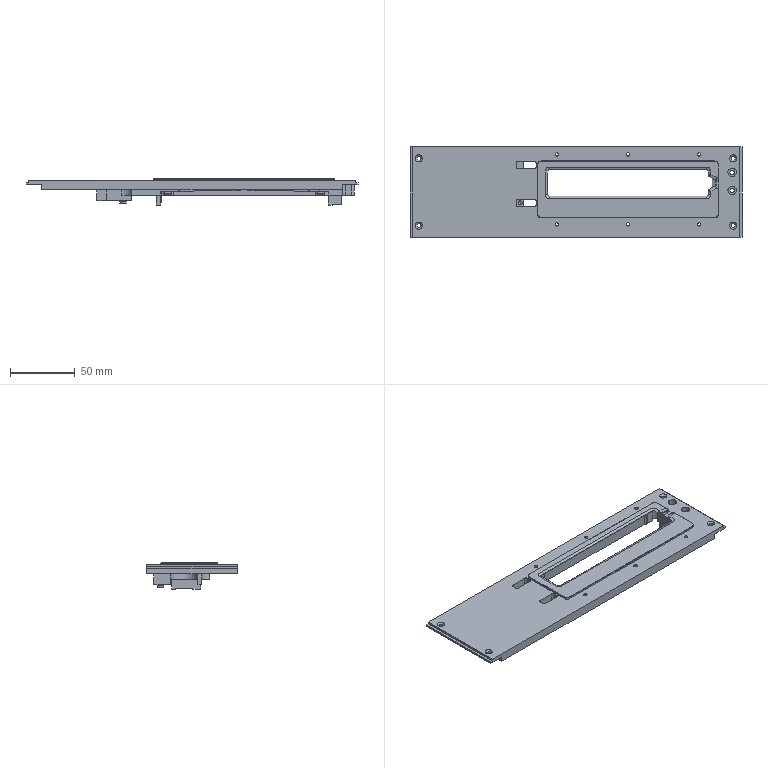NC program | NX | posted with a generic post | part box 256.6 x 70.3 x 20.422 mm
Lines 5836 to 6737 of 23702:
(CAVITY_MILL_COPY_COPY , TOOL : D4)
N11658 T04 M6
N11660 G54
N11662 G17 G0 G90 X21.865 Y-0.04 S9500 M3
N11664 G43 Z30. H4
N11666 Z-0.118
N11668 G94 G1 Z-1.118 F1000.
N11670 G3 X22.479 Y0.418 R1.
N11672 G2 X22.913 Y0.929 R2. F1400.
N11674 G1 Y1.639
N11676 G3 X22.513 Y2.439 R1.
N11678 G1 Z-0.118
N11680 G0 X21.816 Y-0.307 Z-0.32
N11682 G1 Z-1.32 F1000.
N11684 G3 X22.374 Y0.218 R1.
N11686 G2 X22.708 Y0.731 R2. F1400.
N11688 G1 Y1.369
N11690 G3 X22.308 Y2.169 R1.
N11692 G1 Z-0.32
N11694 G0 X21.798 Y-0.624 Z-0.522
N11696 G1 Z-1.522 F1000.
N11698 G3 X22.282 Y-0.03 R1.
N11700 G2 X22.509 Y0.467 R2. F1400.
N11702 G1 Y1.025
N11704 G3 X22.109 Y1.825 R1.
N11706 G1 Z-0.522
N11708 G0 Z30.
N11710 X21.798 Y0.752
N11712 Z-1.322
N11714 G1 Z-2.322 F1000.
N11716 G3 X22.198 Y1.552 R1.
N11718 G1 Y2.15 F1400.
N11720 G2 X21.918 Y2.658 R2.
N11722 G3 X21.396 Y3.218 R1.
N11724 G1 Z-1.322
N11726 G0 X21.798 Y0.752 Z-1.722
N11728 G1 Z-2.722 F1000.
N11730 G3 X22.198 Y1.552 R1.
N11732 G1 Y2.15 F1400.
N11734 G2 X21.918 Y2.658 R2.
N11736 G3 X21.396 Y3.218 R1.
N11738 G1 Z-1.722
N11740 G0 X21.798 Y0.752 Z-2.122
N11742 G1 Z-3.122 F1000.
N11744 G3 X22.198 Y1.552 R1.
N11746 G1 Y2.15 F1400.
N11748 G2 X21.918 Y2.658 R2.
N11750 G3 X21.396 Y3.218 R1.
N11752 G1 Z-2.122
N11754 G0 X21.798 Y0.752 Z-2.522
N11756 G1 Z-3.522 F1000.
N11758 G3 X22.198 Y1.552 R1.
N11760 G1 Y2.15 F1400.
N11762 G2 X21.918 Y2.658 R2.
N11764 G3 X21.396 Y3.218 R1.
N11766 G1 Z-2.522
N11768 G0 X21.798 Y0.752 Z-2.903
N11770 G1 Z-3.903 F1000.
N11772 G3 X22.198 Y1.552 R1.
N11774 G1 Y2.15 F1400.
N11776 G2 X21.918 Y2.658 R2.
N11778 G3 X21.396 Y3.218 R1.
N11780 G1 Z-2.903
N11782 G0 X21.798 Y0.752 Z-3.285
N11784 G1 Z-4.285 F1000.
N11786 G3 X22.198 Y1.552 R1.
N11788 G1 Y2.15 F1400.
N11790 G2 X21.918 Y2.658 R2.
N11792 G3 X21.396 Y3.218 R1.
N11794 G1 Z-3.285
N11796 G0 X21.798 Y0.752 Z-3.667
N11798 G1 Z-4.667 F1000.
N11800 G3 X22.198 Y1.552 R1.
N11802 G1 Y2.15 F1400.
N11804 G2 X21.918 Y2.658 R2.
N11806 G3 X21.396 Y3.218 R1.
N11808 G1 Z-3.667
N11810 G0 X21.798 Y0.752 Z-4.049
N11812 G1 Z-5.049 F1000.
N11814 G3 X22.198 Y1.552 R1.
N11816 G1 Y2.15 F1400.
N11818 G2 X21.918 Y2.658 R2.
N11820 G3 X21.396 Y3.218 R1.
N11822 G1 Z-4.049
N11824 G0 X21.798 Y0.752 Z-4.431
N11826 G1 Z-5.431 F1000.
N11828 G3 X22.198 Y1.552 R1.
N11830 G1 Y2.15 F1400.
N11832 G2 X21.918 Y2.658 R2.
N11834 G3 X21.396 Y3.218 R1.
N11836 G1 Z-4.431
N11838 G0 X21.798 Y0.752 Z-4.813
N11840 G1 Z-5.813 F1000.
N11842 G3 X22.198 Y1.552 R1.
N11844 G1 Y2.15 F1400.
N11846 G2 X21.918 Y2.658 R2.
N11848 G3 X21.396 Y3.218 R1.
N11850 G1 Z-4.813
N11852 G0 X21.798 Y0.752 Z-5.194
N11854 G1 Z-6.194 F1000.
N11856 G3 X22.198 Y1.552 R1.
N11858 G1 Y2.15 F1400.
N11860 G2 X21.918 Y2.658 R2.
N11862 G3 X21.396 Y3.218 R1.
N11864 G1 Z-5.194
N11866 G0 X21.798 Y0.752 Z-5.576
N11868 G1 Z-6.576 F1000.
N11870 G3 X22.198 Y1.552 R1.
N11872 G1 Y2.15 F1400.
N11874 G2 X21.918 Y2.658 R2.
N11876 G3 X21.396 Y3.218 R1.
N11878 G1 Z-5.576
N11880 G0 X21.798 Y0.752 Z-5.958
N11882 G1 Z-6.958 F1000.
N11884 G3 X22.198 Y1.552 R1.
N11886 G1 Y2.15 F1400.
N11888 G2 X21.918 Y2.658 R2.
N11890 G3 X21.396 Y3.218 R1.
N11892 G1 Z-5.958
N11894 G0 X21.798 Y0.752 Z-6.34
N11896 G1 Z-7.34 F1000.
N11898 G3 X22.198 Y1.552 R1.
N11900 G1 Y2.15 F1400.
N11902 G2 X21.918 Y2.658 R2.
N11904 G3 X21.396 Y3.218 R1.
N11906 G1 Z-6.34
N11908 G0 X21.798 Y0.752 Z-6.722
N11910 G1 Z-7.722 F1000.
N11912 G3 X22.198 Y1.552 R1.
N11914 G1 Y2.15 F1400.
N11916 G2 X21.918 Y2.658 R2.
N11918 G3 X21.396 Y3.218 R1.
N11920 G1 Z-6.722
N11922 G0 X21.798 Y0.752 Z-7.092
N11924 G1 Z-8.092 F1000.
N11926 G3 X22.198 Y1.552 R1.
N11928 G1 Y2.15 F1400.
N11930 G2 X21.918 Y2.658 R2.
N11932 G3 X21.396 Y3.218 R1.
N11934 G1 Z-7.092
N11936 G0 X21.798 Y0.752 Z-7.463
N11938 G1 Z-8.463 F1000.
N11940 G3 X22.198 Y1.552 R1.
N11942 G1 Y2.15 F1400.
N11944 G2 X21.918 Y2.658 R2.
N11946 G3 X21.396 Y3.218 R1.
N11948 G1 Z-7.463
N11950 G0 X21.798 Y0.752 Z-7.833
N11952 G1 Z-8.833 F1000.
N11954 G3 X22.198 Y1.552 R1.
N11956 G1 Y2.15 F1400.
N11958 G2 X21.918 Y2.658 R2.
N11960 G3 X21.396 Y3.218 R1.
N11962 G1 Z-7.833
N11964 G0 X21.798 Y0.752 Z-8.204
N11966 G1 Z-9.204 F1000.
N11968 G3 X22.198 Y1.552 R1.
N11970 G1 Y2.15 F1400.
N11972 G2 X21.918 Y2.658 R2.
N11974 G3 X21.396 Y3.218 R1.
N11976 G1 Z-8.204
N11978 G0 X21.798 Y0.752 Z-8.575
N11980 G1 Z-9.575 F1000.
N11982 G3 X22.198 Y1.552 R1.
N11984 G1 Y2.15 F1400.
N11986 G2 X21.918 Y2.658 R2.
N11988 G3 X21.396 Y3.218 R1.
N11990 G1 Z-8.575
N11992 G0 X21.798 Y0.752 Z-8.945
N11994 G1 Z-9.945 F1000.
N11996 G3 X22.198 Y1.552 R1.
N11998 G1 Y2.15 F1400.
N12000 G2 X21.918 Y2.658 R2.
N12002 G3 X21.396 Y3.218 R1.
N12004 G1 Z-8.945
N12006 G0 X21.798 Y0.752 Z-9.316
N12008 G1 Z-10.316 F1000.
N12010 G3 X22.198 Y1.552 R1.
N12012 G1 Y2.15 F1400.
N12014 G2 X21.918 Y2.658 R2.
N12016 G3 X21.396 Y3.218 R1.
N12018 G1 Z-9.316
N12020 G0 X21.798 Y0.752 Z-9.687
N12022 G1 Z-10.687 F1000.
N12024 G3 X22.198 Y1.552 R1.
N12026 G1 Y2.15 F1400.
N12028 G2 X21.918 Y2.658 R2.
N12030 G3 X21.396 Y3.218 R1.
N12032 G1 Z-9.687
N12034 G0 X21.798 Y0.752 Z-10.019
N12036 G1 Z-11.019 F1000.
N12038 G3 X22.198 Y1.552 R1.
N12040 G1 Y2.15 F1400.
N12042 G2 X21.918 Y2.658 R2.
N12044 G3 X21.396 Y3.218 R1.
N12046 G1 Z-10.019
N12048 G0 X21.798 Y0.752 Z-10.27
N12050 G1 Z-11.27 F1000.
N12052 G3 X22.198 Y1.552 R1.
N12054 G1 Y2.15 F1400.
N12056 G2 X21.918 Y2.658 R2.
N12058 G3 X21.396 Y3.218 R1.
N12060 G1 Z-10.27
N12062 G0 X21.798 Y0.752 Z-10.522
N12064 G1 Z-11.522 F1000.
N12066 G3 X22.198 Y1.552 R1.
N12068 G1 Y2.15 F1400.
N12070 G2 X21.918 Y2.658 R2.
N12072 G3 X21.396 Y3.218 R1.
N12074 G1 Z-10.522
N12076 G0 X21.798 Y0.752 Z-10.724
N12078 G1 Z-11.724 F1000.
N12080 G3 X22.198 Y1.552 R1.
N12082 G1 Y2.15 F1400.
N12084 G2 X21.918 Y2.658 R2.
N12086 G3 X21.396 Y3.218 R1.
N12088 G1 Z-10.724
N12090 G0 X21.798 Y0.752 Z-10.925
N12092 G1 Z-11.925 F1000.
N12094 G3 X22.198 Y1.552 R1.
N12096 G1 Y2.15 F1400.
N12098 G2 X21.918 Y2.658 R2.
N12100 G3 X21.396 Y3.218 R1.
N12102 G1 Z-10.925
N12104 G0 X21.798 Y0.752 Z-11.32
N12106 G1 Z-12.32 F1000.
N12108 G3 X22.198 Y1.552 R1.
N12110 G1 Y2.15 F1400.
N12112 G2 X21.918 Y2.658 R2.
N12114 G3 X21.396 Y3.218 R1.
N12116 G1 Z-11.32
N12118 G0 X21.798 Y0.752 Z-11.715
N12120 G1 Z-12.715 F1000.
N12122 G3 X22.198 Y1.552 R1.
N12124 G1 Y2.15 F1400.
N12126 G2 X21.918 Y2.658 R2.
N12128 G3 X21.396 Y3.218 R1.
N12130 G1 Z-11.715
N12132 G0 X21.798 Y0.752 Z-12.109
N12134 G1 Z-13.109 F1000.
N12136 G3 X22.198 Y1.552 R1.
N12138 G1 Y2.15 F1400.
N12140 G2 X21.918 Y2.658 R2.
N12142 G3 X21.396 Y3.218 R1.
N12144 G1 Z-12.109
N12146 G0 X21.798 Y0.752 Z-12.504
N12148 G1 Z-13.504 F1000.
N12150 G3 X22.198 Y1.552 R1.
N12152 G1 Y2.15 F1400.
N12154 G2 X21.918 Y2.658 R2.
N12156 G3 X21.396 Y3.218 R1.
N12158 G1 Z-12.504
N12160 G0 X21.798 Y0.752 Z-12.899
N12162 G1 Z-13.899 F1000.
N12164 G3 X22.198 Y1.552 R1.
N12166 G1 Y2.15 F1400.
N12168 G2 X21.918 Y2.658 R2.
N12170 G3 X21.396 Y3.218 R1.
N12172 G1 Z-12.899
N12174 G0 X21.798 Y0.752 Z-13.293
N12176 G1 Z-14.293 F1000.
N12178 G3 X22.198 Y1.552 R1.
N12180 G1 Y2.15 F1400.
N12182 G2 X21.918 Y2.658 R2.
N12184 G3 X21.396 Y3.218 R1.
N12186 G1 Z-13.293
N12188 G0 X21.798 Y0.752 Z-13.688
N12190 G1 Z-14.688 F1000.
N12192 G3 X22.198 Y1.552 R1.
N12194 G1 Y2.15 F1400.
N12196 G2 X21.918 Y2.658 R2.
N12198 G3 X21.396 Y3.218 R1.
N12200 G1 Z-13.688
N12202 G0 X21.798 Y0.752 Z-14.082
N12204 G1 Z-15.082 F1000.
N12206 G3 X22.198 Y1.552 R1.
N12208 G1 Y2.15 F1400.
N12210 G2 X21.918 Y2.658 R2.
N12212 G3 X21.396 Y3.218 R1.
N12214 G1 Z-14.082
N12216 G0 X21.798 Y0.752 Z-14.477
N12218 G1 Z-15.477 F1000.
N12220 G3 X22.198 Y1.552 R1.
N12222 G1 Y2.15 F1400.
N12224 G2 X21.918 Y2.658 R2.
N12226 G3 X21.396 Y3.218 R1.
N12228 G1 Z-14.477
N12230 G0 X21.798 Y0.752 Z-14.872
N12232 G1 Z-15.872 F1000.
N12234 G3 X22.198 Y1.552 R1.
N12236 G1 Y2.15 F1400.
N12238 G2 X21.918 Y2.658 R2.
N12240 G3 X21.396 Y3.218 R1.
N12242 G1 Z-14.872
N12244 G0 X21.798 Y0.752 Z-14.922
N12246 G1 Z-15.922 F1000.
N12248 G3 X22.198 Y1.552 R1.
N12250 G1 Y2.15 F1400.
N12252 G2 X21.918 Y2.658 R2.
N12254 G3 X21.396 Y3.218 R1.
N12256 G1 Z-14.922
N12258 G0 X21.798 Y0.752 Z-15.222
N12260 G1 Z-16.222 F1000.
N12262 G3 X22.198 Y1.552 R1.
N12264 G1 Y2.15 F1400.
N12266 G2 X21.918 Y2.658 R2.
N12268 G3 X21.396 Y3.218 R1.
N12270 G1 Z-15.222
N12272 G0 X21.798 Y0.752 Z-15.522
N12274 G1 Z-16.522 F1000.
N12276 G3 X22.198 Y1.552 R1.
N12278 G1 Y2.15 F1400.
N12280 G2 X21.918 Y2.658 R2.
N12282 G3 X21.396 Y3.218 R1.
N12284 G1 Z-15.522
N12286 G0 X21.798 Y0.752 Z-15.822
N12288 G1 Z-16.822 F1000.
N12290 G3 X22.198 Y1.552 R1.
N12292 G1 Y2.15 F1400.
N12294 G2 X21.918 Y2.658 R2.
N12296 G3 X21.396 Y3.218 R1.
N12298 G1 Z-15.822
N12300 G0 X21.798 Y0.752 Z-16.179
N12302 G1 Z-17.179 F1000.
N12304 G3 X22.198 Y1.552 R1.
N12306 G1 Y2.15 F1400.
N12308 G2 X21.918 Y2.658 R2.
N12310 G3 X21.396 Y3.218 R1.
N12312 G1 Z-16.179
N12314 G0 X21.798 Y0.752 Z-16.536
N12316 G1 Z-17.536 F1000.
N12318 G3 X22.198 Y1.552 R1.
N12320 G1 Y2.15 F1400.
N12322 G2 X21.918 Y2.658 R2.
N12324 G3 X21.396 Y3.218 R1.
N12326 G1 Z-16.536
N12328 G0 X21.798 Y0.752 Z-16.893
N12330 G1 Z-17.893 F1000.
N12332 G3 X22.198 Y1.552 R1.
N12334 G1 Y2.15 F1400.
N12336 G2 X21.918 Y2.658 R2.
N12338 G3 X21.396 Y3.218 R1.
N12340 G1 Z-16.893
N12342 G0 X21.798 Y0.752 Z-17.25
N12344 G1 Z-18.25 F1000.
N12346 G3 X22.198 Y1.552 R1.
N12348 G1 Y2.15 F1400.
N12350 G2 X21.918 Y2.658 R2.
N12352 G3 X21.396 Y3.218 R1.
N12354 G1 Z-17.25
N12356 G0 X21.798 Y0.752 Z-17.607
N12358 G1 Z-18.607 F1000.
N12360 G3 X22.198 Y1.552 R1.
N12362 G1 Y2.15 F1400.
N12364 G2 X21.918 Y2.658 R2.
N12366 G3 X21.396 Y3.218 R1.
N12368 G1 Z-17.607
N12370 G0 X21.798 Y0.752 Z-17.964
N12372 G1 Z-18.964 F1000.
N12374 G3 X22.198 Y1.552 R1.
N12376 G1 Y2.15 F1400.
N12378 G2 X21.918 Y2.658 R2.
N12380 G3 X21.396 Y3.218 R1.
N12382 G1 Z-17.964
N12384 G0 X21.798 Y0.752 Z-18.322
N12386 G1 Z-19.322 F1000.
N12388 G3 X22.198 Y1.552 R1.
N12390 G1 Y2.15 F1400.
N12392 G2 X21.918 Y2.658 R2.
N12394 G3 X21.396 Y3.218 R1.
N12396 G1 Z-18.322
N12398 G0 Z30.
N12400 X22.513 Y9.561
N12402 Z-0.118
N12404 G1 Z-1.118 F1000.
N12406 G3 X22.913 Y10.361 R1.
N12408 G1 Y11.071 F1400.
N12410 G2 X22.479 Y11.582 R2.
N12412 G3 X21.865 Y12.04 R1.
N12414 G1 Z-0.118
N12416 G0 X22.308 Y9.831 Z-0.32
N12418 G1 Z-1.32 F1000.
N12420 G3 X22.708 Y10.631 R1.
N12422 G1 Y11.269 F1400.
N12424 G2 X22.374 Y11.782 R2.
N12426 G3 X21.816 Y12.307 R1.
N12428 G1 Z-0.32
N12430 G0 X22.109 Y10.175 Z-0.522
N12432 G1 Z-1.522 F1000.
N12434 G3 X22.509 Y10.975 R1.
N12436 G1 Y11.533 F1400.
N12438 G2 X22.282 Y12.03 R2.
N12440 G3 X21.798 Y12.624 R1.
N12442 G1 Z-0.522
N12444 G0 Z30.
N12446 X21.396 Y8.782
N12448 Z-1.322
N12450 G1 Z-2.322 F1000.
N12452 G3 X21.918 Y9.342 R1.
N12454 G2 X22.198 Y9.85 R2. F1400.
N12456 G1 Y10.448
N12458 G3 X21.798 Y11.248 R1.
N12460 G1 Z-1.322
N12462 G0 X21.396 Y8.782 Z-1.722
N12464 G1 Z-2.722 F1000.
N12466 G3 X21.918 Y9.342 R1.
N12468 G2 X22.198 Y9.85 R2. F1400.
N12470 G1 Y10.448
N12472 G3 X21.798 Y11.248 R1.
N12474 G1 Z-1.722
N12476 G0 X21.396 Y8.782 Z-2.122
N12478 G1 Z-3.122 F1000.
N12480 G3 X21.918 Y9.342 R1.
N12482 G2 X22.198 Y9.85 R2. F1400.
N12484 G1 Y10.448
N12486 G3 X21.798 Y11.248 R1.
N12488 G1 Z-2.122
N12490 G0 X21.396 Y8.782 Z-2.522
N12492 G1 Z-3.522 F1000.
N12494 G3 X21.918 Y9.342 R1.
N12496 G2 X22.198 Y9.85 R2. F1400.
N12498 G1 Y10.448
N12500 G3 X21.798 Y11.248 R1.
N12502 G1 Z-2.522
N12504 G0 X21.396 Y8.782 Z-2.903
N12506 G1 Z-3.903 F1000.
N12508 G3 X21.918 Y9.342 R1.
N12510 G2 X22.198 Y9.85 R2. F1400.
N12512 G1 Y10.448
N12514 G3 X21.798 Y11.248 R1.
N12516 G1 Z-2.903
N12518 G0 X21.396 Y8.782 Z-3.285
N12520 G1 Z-4.285 F1000.
N12522 G3 X21.918 Y9.342 R1.
N12524 G2 X22.198 Y9.85 R2. F1400.
N12526 G1 Y10.448
N12528 G3 X21.798 Y11.248 R1.
N12530 G1 Z-3.285
N12532 G0 X21.396 Y8.782 Z-3.667
N12534 G1 Z-4.667 F1000.
N12536 G3 X21.918 Y9.342 R1.
N12538 G2 X22.198 Y9.85 R2. F1400.
N12540 G1 Y10.448
N12542 G3 X21.798 Y11.248 R1.
N12544 G1 Z-3.667
N12546 G0 X21.396 Y8.782 Z-4.049
N12548 G1 Z-5.049 F1000.
N12550 G3 X21.918 Y9.342 R1.
N12552 G2 X22.198 Y9.85 R2. F1400.
N12554 G1 Y10.448
N12556 G3 X21.798 Y11.248 R1.
N12558 G1 Z-4.049
N12560 G0 X21.396 Y8.782 Z-4.431
N12562 G1 Z-5.431 F1000.
N12564 G3 X21.918 Y9.342 R1.
N12566 G2 X22.198 Y9.85 R2. F1400.
N12568 G1 Y10.448
N12570 G3 X21.798 Y11.248 R1.
N12572 G1 Z-4.431
N12574 G0 X21.396 Y8.782 Z-4.813
N12576 G1 Z-5.813 F1000.
N12578 G3 X21.918 Y9.342 R1.
N12580 G2 X22.198 Y9.85 R2. F1400.
N12582 G1 Y10.448
N12584 G3 X21.798 Y11.248 R1.
N12586 G1 Z-4.813
N12588 G0 X21.396 Y8.782 Z-5.194
N12590 G1 Z-6.194 F1000.
N12592 G3 X21.918 Y9.342 R1.
N12594 G2 X22.198 Y9.85 R2. F1400.
N12596 G1 Y10.448
N12598 G3 X21.798 Y11.248 R1.
N12600 G1 Z-5.194
N12602 G0 X21.396 Y8.782 Z-5.576
N12604 G1 Z-6.576 F1000.
N12606 G3 X21.918 Y9.342 R1.
N12608 G2 X22.198 Y9.85 R2. F1400.
N12610 G1 Y10.448
N12612 G3 X21.798 Y11.248 R1.
N12614 G1 Z-5.576
N12616 G0 X21.396 Y8.782 Z-5.958
N12618 G1 Z-6.958 F1000.
N12620 G3 X21.918 Y9.342 R1.
N12622 G2 X22.198 Y9.85 R2. F1400.
N12624 G1 Y10.448
N12626 G3 X21.798 Y11.248 R1.
N12628 G1 Z-5.958
N12630 G0 X21.396 Y8.782 Z-6.34
N12632 G1 Z-7.34 F1000.
N12634 G3 X21.918 Y9.342 R1.
N12636 G2 X22.198 Y9.85 R2. F1400.
N12638 G1 Y10.448
N12640 G3 X21.798 Y11.248 R1.
N12642 G1 Z-6.34
N12644 G0 X21.396 Y8.782 Z-6.722
N12646 G1 Z-7.722 F1000.
N12648 G3 X21.918 Y9.342 R1.
N12650 G2 X22.198 Y9.85 R2. F1400.
N12652 G1 Y10.448
N12654 G3 X21.798 Y11.248 R1.
N12656 G1 Z-6.722
N12658 G0 X21.396 Y8.782 Z-7.092
N12660 G1 Z-8.092 F1000.
N12662 G3 X21.918 Y9.342 R1.
N12664 G2 X22.198 Y9.85 R2. F1400.
N12666 G1 Y10.448
N12668 G3 X21.798 Y11.248 R1.
N12670 G1 Z-7.092
N12672 G0 X21.396 Y8.782 Z-7.463
N12674 G1 Z-8.463 F1000.
N12676 G3 X21.918 Y9.342 R1.
N12678 G2 X22.198 Y9.85 R2. F1400.
N12680 G1 Y10.448
N12682 G3 X21.798 Y11.248 R1.
N12684 G1 Z-7.463
N12686 G0 X21.396 Y8.782 Z-7.833
N12688 G1 Z-8.833 F1000.
N12690 G3 X21.918 Y9.342 R1.
N12692 G2 X22.198 Y9.85 R2. F1400.
N12694 G1 Y10.448
N12696 G3 X21.798 Y11.248 R1.
N12698 G1 Z-7.833
N12700 G0 X21.396 Y8.782 Z-8.204
N12702 G1 Z-9.204 F1000.
N12704 G3 X21.918 Y9.342 R1.
N12706 G2 X22.198 Y9.85 R2. F1400.
N12708 G1 Y10.448
N12710 G3 X21.798 Y11.248 R1.
N12712 G1 Z-8.204
N12714 G0 X21.396 Y8.782 Z-8.575
N12716 G1 Z-9.575 F1000.
N12718 G3 X21.918 Y9.342 R1.
N12720 G2 X22.198 Y9.85 R2. F1400.
N12722 G1 Y10.448
N12724 G3 X21.798 Y11.248 R1.
N12726 G1 Z-8.575
N12728 G0 X21.396 Y8.782 Z-8.945
N12730 G1 Z-9.945 F1000.
N12732 G3 X21.918 Y9.342 R1.
N12734 G2 X22.198 Y9.85 R2. F1400.
N12736 G1 Y10.448
N12738 G3 X21.798 Y11.248 R1.
N12740 G1 Z-8.945
N12742 G0 X21.396 Y8.782 Z-9.316
N12744 G1 Z-10.316 F1000.
N12746 G3 X21.918 Y9.342 R1.
N12748 G2 X22.198 Y9.85 R2. F1400.
N12750 G1 Y10.448
N12752 G3 X21.798 Y11.248 R1.
N12754 G1 Z-9.316
N12756 G0 X21.396 Y8.782 Z-9.687
N12758 G1 Z-10.687 F1000.
N12760 G3 X21.918 Y9.342 R1.
N12762 G2 X22.198 Y9.85 R2. F1400.
N12764 G1 Y10.448
N12766 G3 X21.798 Y11.248 R1.
N12768 G1 Z-9.687
N12770 G0 X21.396 Y8.782 Z-10.019
N12772 G1 Z-11.019 F1000.
N12774 G3 X21.918 Y9.342 R1.
N12776 G2 X22.198 Y9.85 R2. F1400.
N12778 G1 Y10.448
N12780 G3 X21.798 Y11.248 R1.
N12782 G1 Z-10.019
N12784 G0 X21.396 Y8.782 Z-10.27
N12786 G1 Z-11.27 F1000.
N12788 G3 X21.918 Y9.342 R1.
N12790 G2 X22.198 Y9.85 R2. F1400.
N12792 G1 Y10.448
N12794 G3 X21.798 Y11.248 R1.
N12796 G1 Z-10.27
N12798 G0 X21.396 Y8.782 Z-10.522
N12800 G1 Z-11.522 F1000.
N12802 G3 X21.918 Y9.342 R1.
N12804 G2 X22.198 Y9.85 R2. F1400.
N12806 G1 Y10.448
N12808 G3 X21.798 Y11.248 R1.
N12810 G1 Z-10.522
N12812 G0 X21.396 Y8.782 Z-10.724
N12814 G1 Z-11.724 F1000.
N12816 G3 X21.918 Y9.342 R1.
N12818 G2 X22.198 Y9.85 R2. F1400.
N12820 G1 Y10.448
N12822 G3 X21.798 Y11.248 R1.
N12824 G1 Z-10.724
N12826 G0 X21.396 Y8.782 Z-10.925
N12828 G1 Z-11.925 F1000.
N12830 G3 X21.918 Y9.342 R1.
N12832 G2 X22.198 Y9.85 R2. F1400.
N12834 G1 Y10.448
N12836 G3 X21.798 Y11.248 R1.
N12838 G1 Z-10.925
N12840 G0 X21.396 Y8.782 Z-11.32
N12842 G1 Z-12.32 F1000.
N12844 G3 X21.918 Y9.342 R1.
N12846 G2 X22.198 Y9.85 R2. F1400.
N12848 G1 Y10.448
N12850 G3 X21.798 Y11.248 R1.
N12852 G1 Z-11.32
N12854 G0 X21.396 Y8.782 Z-11.715
N12856 G1 Z-12.715 F1000.
N12858 G3 X21.918 Y9.342 R1.
N12860 G2 X22.198 Y9.85 R2. F1400.
N12862 G1 Y10.448
N12864 G3 X21.798 Y11.248 R1.
N12866 G1 Z-11.715
N12868 G0 X21.396 Y8.782 Z-12.109
N12870 G1 Z-13.109 F1000.
N12872 G3 X21.918 Y9.342 R1.
N12874 G2 X22.198 Y9.85 R2. F1400.
N12876 G1 Y10.448
N12878 G3 X21.798 Y11.248 R1.
N12880 G1 Z-12.109
N12882 G0 X21.396 Y8.782 Z-12.504
N12884 G1 Z-13.504 F1000.
N12886 G3 X21.918 Y9.342 R1.
N12888 G2 X22.198 Y9.85 R2. F1400.
N12890 G1 Y10.448
N12892 G3 X21.798 Y11.248 R1.
N12894 G1 Z-12.504
N12896 G0 X21.396 Y8.782 Z-12.899
N12898 G1 Z-13.899 F1000.
N12900 G3 X21.918 Y9.342 R1.
N12902 G2 X22.198 Y9.85 R2. F1400.
N12904 G1 Y10.448
N12906 G3 X21.798 Y11.248 R1.
N12908 G1 Z-12.899
N12910 G0 X21.396 Y8.782 Z-13.293
N12912 G1 Z-14.293 F1000.
N12914 G3 X21.918 Y9.342 R1.
N12916 G2 X22.198 Y9.85 R2. F1400.
N12918 G1 Y10.448
N12920 G3 X21.798 Y11.248 R1.
N12922 G1 Z-13.293
N12924 G0 X21.396 Y8.782 Z-13.688
N12926 G1 Z-14.688 F1000.
N12928 G3 X21.918 Y9.342 R1.
N12930 G2 X22.198 Y9.85 R2. F1400.
N12932 G1 Y10.448
N12934 G3 X21.798 Y11.248 R1.
N12936 G1 Z-13.688
N12938 G0 X21.396 Y8.782 Z-14.082
N12940 G1 Z-15.082 F1000.
N12942 G3 X21.918 Y9.342 R1.
N12944 G2 X22.198 Y9.85 R2. F1400.
N12946 G1 Y10.448
N12948 G3 X21.798 Y11.248 R1.
N12950 G1 Z-14.082
N12952 G0 X21.396 Y8.782 Z-14.477
N12954 G1 Z-15.477 F1000.
N12956 G3 X21.918 Y9.342 R1.
N12958 G2 X22.198 Y9.85 R2. F1400.
N12960 G1 Y10.448
N12962 G3 X21.798 Y11.248 R1.
N12964 G1 Z-14.477
N12966 G0 X21.396 Y8.782 Z-14.872
N12968 G1 Z-15.872 F1000.
N12970 G3 X21.918 Y9.342 R1.
N12972 G2 X22.198 Y9.85 R2. F1400.
N12974 G1 Y10.448
N12976 G3 X21.798 Y11.248 R1.
N12978 G1 Z-14.872
N12980 G0 X21.396 Y8.782 Z-14.922
N12982 G1 Z-15.922 F1000.
N12984 G3 X21.918 Y9.342 R1.
N12986 G2 X22.198 Y9.85 R2. F1400.
N12988 G1 Y10.448
N12990 G3 X21.798 Y11.248 R1.
N12992 G1 Z-14.922
N12994 G0 X21.396 Y8.782 Z-15.222
N12996 G1 Z-16.222 F1000.
N12998 G3 X21.918 Y9.342 R1.
N13000 G2 X22.198 Y9.85 R2. F1400.
N13002 G1 Y10.448
N13004 G3 X21.798 Y11.248 R1.
N13006 G1 Z-15.222
N13008 G0 X21.396 Y8.782 Z-15.522
N13010 G1 Z-16.522 F1000.
N13012 G3 X21.918 Y9.342 R1.
N13014 G2 X22.198 Y9.85 R2. F1400.
N13016 G1 Y10.448
N13018 G3 X21.798 Y11.248 R1.
N13020 G1 Z-15.522
N13022 G0 X21.396 Y8.782 Z-15.822
N13024 G1 Z-16.822 F1000.
N13026 G3 X21.918 Y9.342 R1.
N13028 G2 X22.198 Y9.85 R2. F1400.
N13030 G1 Y10.448
N13032 G3 X21.798 Y11.248 R1.
N13034 G1 Z-15.822
N13036 G0 X21.396 Y8.782 Z-16.179
N13038 G1 Z-17.179 F1000.
N13040 G3 X21.918 Y9.342 R1.
N13042 G2 X22.198 Y9.85 R2. F1400.
N13044 G1 Y10.448
N13046 G3 X21.798 Y11.248 R1.
N13048 G1 Z-16.179
N13050 G0 X21.396 Y8.782 Z-16.536
N13052 G1 Z-17.536 F1000.
N13054 G3 X21.918 Y9.342 R1.
N13056 G2 X22.198 Y9.85 R2. F1400.
N13058 G1 Y10.448
N13060 G3 X21.798 Y11.248 R1.
N13062 G1 Z-16.536
N13064 G0 X21.396 Y8.782 Z-16.893
N13066 G1 Z-17.893 F1000.
N13068 G3 X21.918 Y9.342 R1.
N13070 G2 X22.198 Y9.85 R2. F1400.
N13072 G1 Y10.448
N13074 G3 X21.798 Y11.248 R1.
N13076 G1 Z-16.893
N13078 G0 X21.396 Y8.782 Z-17.25
N13080 G1 Z-18.25 F1000.
N13082 G3 X21.918 Y9.342 R1.
N13084 G2 X22.198 Y9.85 R2. F1400.
N13086 G1 Y10.448
N13088 G3 X21.798 Y11.248 R1.
N13090 G1 Z-17.25
N13092 G0 X21.396 Y8.782 Z-17.607
N13094 G1 Z-18.607 F1000.
N13096 G3 X21.918 Y9.342 R1.
N13098 G2 X22.198 Y9.85 R2. F1400.
N13100 G1 Y10.448
N13102 G3 X21.798 Y11.248 R1.
N13104 G1 Z-17.607
N13106 G0 X21.396 Y8.782 Z-17.964
N13108 G1 Z-18.964 F1000.
N13110 G3 X21.918 Y9.342 R1.
N13112 G2 X22.198 Y9.85 R2. F1400.
N13114 G1 Y10.448
N13116 G3 X21.798 Y11.248 R1.
N13118 G1 Z-17.964
N13120 G0 X21.396 Y8.782 Z-18.322
N13122 G1 Z-19.322 F1000.
N13124 G3 X21.918 Y9.342 R1.
N13126 G2 X22.198 Y9.85 R2. F1400.
N13128 G1 Y10.448
N13130 G3 X21.798 Y11.248 R1.
N13132 G1 Z-18.322
N13134 G0 Z30.
N13136 Y15.499
N13138 Z-7.092
N13140 G1 Z-8.092 F1000.
N13142 G3 X22.245 Y16.131 R1.
N13144 G2 X24.198 Y17.7 R2. F1400.
N13146 G3 X23.272 Y19.077 R-1.
N13148 G2 X21.421 Y17.829 R1.987
N13150 G1 X21.085
N13152 G3 X20.285 Y17.429 R1.
N13154 G1 Z-7.092
N13156 G0 X21.798 Y15.153 Z-7.463
N13158 G1 Z-8.463 F1000.
N13160 G3 X22.205 Y15.874 R1.
N13162 G2 X24.198 Y17.7 R2. F1400.
N13164 G3 X23.23 Y18.953 R-1.
N13166 G2 X21.3 Y17.459 R1.998
N13168 G1 X20.96
N13170 G3 X20.16 Y17.059 R1.
N13172 G1 Z-7.463
N13174 G0 X21.798 Y14.823 Z-7.833
N13176 G1 Z-8.833 F1000.
N13178 G3 X22.198 Y15.623 R1.
N13180 G1 Y15.7 F1400.
N13182 G2 X24.198 Y17.7 R2.
N13184 G3 X23.206 Y18.829 R-1.
N13186 G2 X21.224 Y17.088 R1.999
N13188 G1 X20.887
N13190 G3 X20.087 Y16.688 R1.
N13192 G1 Z-7.833
N13194 G0 X21.798 Y14.576 Z-8.204
N13196 G1 Z-9.204 F1000.
N13198 G3 X22.198 Y15.376 R1.
N13200 G1 Y15.7 F1400.
N13202 G2 X24.198 Y17.7 R2.
N13204 G3 X23.198 Y18.706 R-1.
N13206 G2 X21.199 Y16.718 R2.
N13208 G1 X20.862
N13210 G3 X20.062 Y16.318 R1.
N13212 G1 Z-8.204
N13214 G0 X21.798 Y14.564 Z-8.575
N13216 G1 Z-9.575 F1000.
N13218 G3 X22.198 Y15.364 R1.
N13220 G1 Y15.7 F1400.
N13222 G2 X24.198 Y17.7 R2.
N13224 G3 X23.198 Y18.7 R-1.
N13226 G2 X21.198 Y16.7 R2.
N13228 G1 X20.862
N13230 G3 X20.062 Y16.3 R1.
N13232 G1 Z-8.575
N13234 G0 X21.798 Y14.564 Z-8.945
N13236 G1 Z-9.945 F1000.
N13238 G3 X22.198 Y15.364 R1.
N13240 G1 Y15.7 F1400.
N13242 G2 X24.198 Y17.7 R2.
N13244 G3 X23.198 Y18.7 R-1.
N13246 G2 X21.198 Y16.7 R2.
N13248 G1 X20.862
N13250 G3 X20.062 Y16.3 R1.
N13252 G1 Z-8.945
N13254 G0 X21.798 Y14.564 Z-9.316
N13256 G1 Z-10.316 F1000.
N13258 G3 X22.198 Y15.364 R1.
N13260 G1 Y15.7 F1400.
N13262 G2 X24.198 Y17.7 R2.
N13264 G3 X23.198 Y18.7 R-1.
N13266 G2 X21.198 Y16.7 R2.
N13268 G1 X20.862
N13270 G3 X20.062 Y16.3 R1.
N13272 G1 Z-9.316
N13274 G0 X21.798 Y14.564 Z-9.687
N13276 G1 Z-10.687 F1000.
N13278 G3 X22.198 Y15.364 R1.
N13280 G1 Y15.7 F1400.
N13282 G2 X24.198 Y17.7 R2.
N13284 G3 X23.198 Y18.7 R-1.
N13286 G2 X21.198 Y16.7 R2.
N13288 G1 X20.862
N13290 G3 X20.062 Y16.3 R1.
N13292 G1 Z-9.687
N13294 G0 X21.798 Y14.564 Z-10.019
N13296 G1 Z-11.019 F1000.
N13298 G3 X22.198 Y15.364 R1.
N13300 G1 Y15.7 F1400.
N13302 G2 X24.198 Y17.7 R2.
N13304 G3 X23.198 Y18.7 R-1.
N13306 G2 X21.198 Y16.7 R2.
N13308 G1 X20.862
N13310 G3 X20.062 Y16.3 R1.
N13312 G1 Z-10.019
N13314 G0 X21.798 Y14.564 Z-10.27
N13316 G1 Z-11.27 F1000.
N13318 G3 X22.198 Y15.364 R1.
N13320 G1 Y15.7 F1400.
N13322 G2 X24.198 Y17.7 R2.
N13324 G3 X23.198 Y18.7 R-1.
N13326 G2 X21.198 Y16.7 R2.
N13328 G1 X20.862
N13330 G3 X20.062 Y16.3 R1.
N13332 G1 Z-10.27
N13334 G0 X21.798 Y14.564 Z-10.522
N13336 G1 Z-11.522 F1000.
N13338 G3 X22.198 Y15.364 R1.
N13340 G1 Y15.7 F1400.
N13342 G2 X24.198 Y17.7 R2.
N13344 G3 X23.198 Y18.7 R-1.
N13346 G2 X21.198 Y16.7 R2.
N13348 G1 X20.862
N13350 G3 X20.062 Y16.3 R1.
N13352 G1 Z-10.522
N13354 G0 X21.798 Y14.564 Z-10.724
N13356 G1 Z-11.724 F1000.
N13358 G3 X22.198 Y15.364 R1.
N13360 G1 Y15.7 F1400.
N13362 G2 X24.198 Y17.7 R2.
N13364 G3 X23.198 Y18.7 R-1.
N13366 G2 X21.198 Y16.7 R2.
N13368 G1 X20.862
N13370 G3 X20.062 Y16.3 R1.
N13372 G1 Z-10.724
N13374 G0 X21.798 Y14.564 Z-10.925
N13376 G1 Z-11.925 F1000.
N13378 G3 X22.198 Y15.364 R1.
N13380 G1 Y15.7 F1400.
N13382 G2 X24.198 Y17.7 R2.
N13384 G3 X23.198 Y18.7 R-1.
N13386 G2 X21.198 Y16.7 R2.
N13388 G1 X20.862
N13390 G3 X20.062 Y16.3 R1.
N13392 G1 Z-10.925
N13394 G0 X21.798 Y14.564 Z-11.32
N13396 G1 Z-12.32 F1000.
N13398 G3 X22.198 Y15.364 R1.
N13400 G1 Y15.7 F1400.
N13402 G2 X24.198 Y17.7 R2.
N13404 G3 X23.198 Y18.7 R-1.
N13406 G2 X21.198 Y16.7 R2.
N13408 G1 X20.862
N13410 G3 X20.062 Y16.3 R1.
N13412 G1 Z-11.32
N13414 G0 X21.798 Y14.564 Z-11.715
N13416 G1 Z-12.715 F1000.
N13418 G3 X22.198 Y15.364 R1.
N13420 G1 Y15.7 F1400.
N13422 G2 X24.198 Y17.7 R2.
N13424 G3 X23.198 Y18.7 R-1.
N13426 G2 X21.198 Y16.7 R2.
N13428 G1 X20.862
N13430 G3 X20.062 Y16.3 R1.
N13432 G1 Z-11.715
N13434 G0 X21.798 Y14.564 Z-12.109
N13436 G1 Z-13.109 F1000.
N13438 G3 X22.198 Y15.364 R1.
N13440 G1 Y15.7 F1400.
N13442 G2 X24.198 Y17.7 R2.
N13444 G3 X23.198 Y18.7 R-1.
N13446 G2 X21.198 Y16.7 R2.
N13448 G1 X20.862
N13450 G3 X20.062 Y16.3 R1.
N13452 G1 Z-12.109
N13454 G0 X21.798 Y14.564 Z-12.504